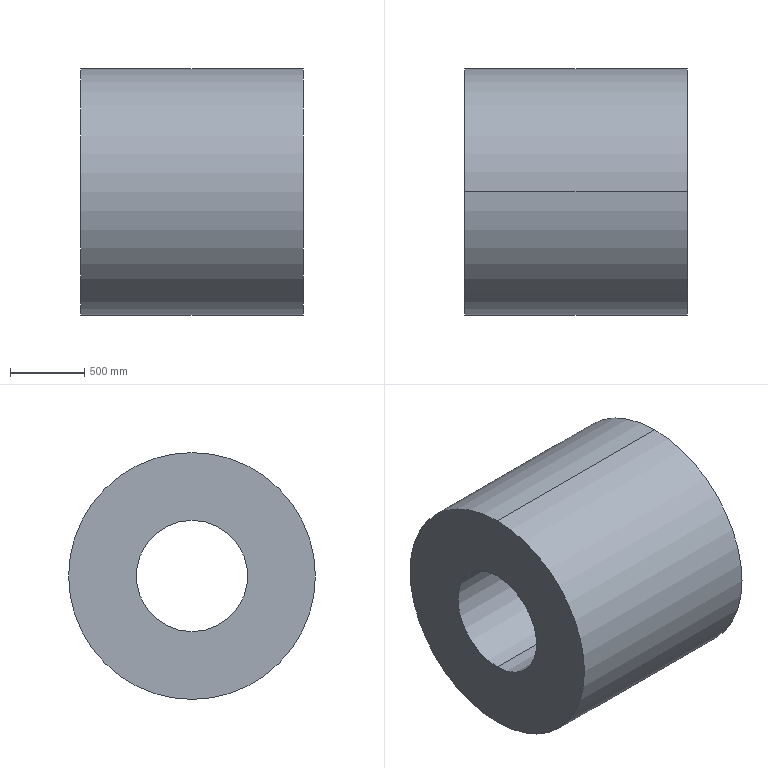Part | SolidWorks | features Extrusion 1 | 1 solid | 6 faces | box 1500 x 1660 x 1660 mm | volume 2583685068 mm3 | cylinder 4 | plane 2 | commonest cylinder face diameters 750 x2 1660 x2
STEP:
#1=CARTESIAN_POINT('',(1500.,0.,375.));
#2=VERTEX_POINT('',#1);
#3=CARTESIAN_POINT('',(1500.,0.,-375.));
#4=VERTEX_POINT('',#3);
#5=CARTESIAN_POINT('',(1500.,0.,0.));
#6=DIRECTION('',(1.,0.,0.));
#7=DIRECTION('',(0.,0.,-1.));
#8=AXIS2_PLACEMENT_3D('',#5,#6,#7);
#9=CIRCLE('',#8,375.);
#10=EDGE_CURVE('',#2,#4,#9,.T.);
#11=ORIENTED_EDGE('',*,*,#10,.T.);
#12=CARTESIAN_POINT('',(0.,0.,-375.));
#13=VERTEX_POINT('',#12);
#14=CARTESIAN_POINT('',(1500.,0.,-375.));
#15=DIRECTION('',(-1.,0.,0.));
#16=VECTOR('',#15,1000.);
#17=LINE('',#14,#16);
#18=EDGE_CURVE('',#4,#13,#17,.T.);
#19=ORIENTED_EDGE('',*,*,#18,.T.);
#20=CARTESIAN_POINT('',(0.,0.,375.));
#21=VERTEX_POINT('',#20);
#22=CARTESIAN_POINT('',(0.,0.,0.));
#23=DIRECTION('',(1.,0.,0.));
#24=DIRECTION('',(0.,0.,-1.));
#25=AXIS2_PLACEMENT_3D('',#22,#23,#24);
#26=CIRCLE('',#25,375.);
#27=EDGE_CURVE('',#21,#13,#26,.T.);
#28=ORIENTED_EDGE('',*,*,#27,.F.);
#29=CARTESIAN_POINT('',(1500.,0.,375.));
#30=DIRECTION('',(-1.,0.,0.));
#31=VECTOR('',#30,1000.);
#32=LINE('',#29,#31);
#33=EDGE_CURVE('',#2,#21,#32,.T.);
#34=ORIENTED_EDGE('',*,*,#33,.F.);
#35=EDGE_LOOP('',(#11,#19,#28,#34));
#36=FACE_OUTER_BOUND('',#35,.T.);
#37=CARTESIAN_POINT('',(1500.,0.,0.));
#38=DIRECTION('',(-1.,0.,0.));
#39=DIRECTION('',(0.,0.,1.));
#40=AXIS2_PLACEMENT_3D('',#37,#38,#39);
#41=CYLINDRICAL_SURFACE('',#40,375.);
#42=ADVANCED_FACE('',(#36),#41,.F.);
#43=CARTESIAN_POINT('',(1500.,0.,-830.));
#44=VERTEX_POINT('',#43);
#45=CARTESIAN_POINT('',(1500.,0.,830.));
#46=VERTEX_POINT('',#45);
#47=CARTESIAN_POINT('',(1500.,0.,0.));
#48=DIRECTION('',(1.,0.,0.));
#49=DIRECTION('',(0.,0.,-1.));
#50=AXIS2_PLACEMENT_3D('',#47,#48,#49);
#51=CIRCLE('',#50,830.);
#52=EDGE_CURVE('',#44,#46,#51,.T.);
#53=ORIENTED_EDGE('',*,*,#52,.F.);
#54=CARTESIAN_POINT('',(0.,0.,-830.));
#55=VERTEX_POINT('',#54);
#56=CARTESIAN_POINT('',(1500.,0.,-830.));
#57=DIRECTION('',(-1.,0.,0.));
#58=VECTOR('',#57,1000.);
#59=LINE('',#56,#58);
#60=EDGE_CURVE('',#44,#55,#59,.T.);
#61=ORIENTED_EDGE('',*,*,#60,.T.);
#62=CARTESIAN_POINT('',(0.,0.,830.));
#63=VERTEX_POINT('',#62);
#64=CARTESIAN_POINT('',(0.,0.,0.));
#65=DIRECTION('',(1.,0.,0.));
#66=DIRECTION('',(0.,0.,-1.));
#67=AXIS2_PLACEMENT_3D('',#64,#65,#66);
#68=CIRCLE('',#67,830.);
#69=EDGE_CURVE('',#55,#63,#68,.T.);
#70=ORIENTED_EDGE('',*,*,#69,.T.);
#71=CARTESIAN_POINT('',(1500.,0.,830.));
#72=DIRECTION('',(-1.,0.,0.));
#73=VECTOR('',#72,1000.);
#74=LINE('',#71,#73);
#75=EDGE_CURVE('',#46,#63,#74,.T.);
#76=ORIENTED_EDGE('',*,*,#75,.F.);
#77=EDGE_LOOP('',(#53,#61,#70,#76));
#78=FACE_OUTER_BOUND('',#77,.T.);
#79=CARTESIAN_POINT('',(1500.,0.,0.));
#80=DIRECTION('',(-1.,0.,0.));
#81=DIRECTION('',(0.,0.,1.));
#82=AXIS2_PLACEMENT_3D('',#79,#80,#81);
#83=CYLINDRICAL_SURFACE('',#82,830.);
#84=ADVANCED_FACE('',(#78),#83,.T.);
#85=CARTESIAN_POINT('',(1500.,0.,0.));
#86=DIRECTION('',(1.,0.,0.));
#87=DIRECTION('',(0.,0.,-1.));
#88=AXIS2_PLACEMENT_3D('',#85,#86,#87);
#89=CIRCLE('',#88,830.);
#90=EDGE_CURVE('',#46,#44,#89,.T.);
#91=ORIENTED_EDGE('',*,*,#90,.T.);
#92=ORIENTED_EDGE('',*,*,#52,.T.);
#93=EDGE_LOOP('',(#91,#92));
#94=FACE_OUTER_BOUND('',#93,.T.);
#95=ORIENTED_EDGE('',*,*,#10,.F.);
#96=CARTESIAN_POINT('',(1500.,0.,0.));
#97=DIRECTION('',(1.,0.,0.));
#98=DIRECTION('',(0.,0.,-1.));
#99=AXIS2_PLACEMENT_3D('',#96,#97,#98);
#100=CIRCLE('',#99,375.);
#101=EDGE_CURVE('',#4,#2,#100,.T.);
#102=ORIENTED_EDGE('',*,*,#101,.F.);
#103=EDGE_LOOP('',(#95,#102));
#104=FACE_BOUND('',#103,.T.);
#105=CARTESIAN_POINT('',(1500.,0.,0.));
#106=DIRECTION('',(1.,0.,0.));
#107=DIRECTION('',(0.,0.,-1.));
#108=AXIS2_PLACEMENT_3D('',#105,#106,#107);
#109=PLANE('',#108);
#110=ADVANCED_FACE('',(#94,#104),#109,.T.);
#111=CARTESIAN_POINT('',(0.,0.,0.));
#112=DIRECTION('',(1.,0.,0.));
#113=DIRECTION('',(0.,0.,-1.));
#114=AXIS2_PLACEMENT_3D('',#111,#112,#113);
#115=CIRCLE('',#114,830.);
#116=EDGE_CURVE('',#63,#55,#115,.T.);
#117=ORIENTED_EDGE('',*,*,#116,.F.);
#118=ORIENTED_EDGE('',*,*,#69,.F.);
#119=EDGE_LOOP('',(#117,#118));
#120=FACE_OUTER_BOUND('',#119,.T.);
#121=ORIENTED_EDGE('',*,*,#27,.T.);
#122=CARTESIAN_POINT('',(0.,0.,0.));
#123=DIRECTION('',(1.,0.,0.));
#124=DIRECTION('',(0.,0.,-1.));
#125=AXIS2_PLACEMENT_3D('',#122,#123,#124);
#126=CIRCLE('',#125,375.);
#127=EDGE_CURVE('',#13,#21,#126,.T.);
#128=ORIENTED_EDGE('',*,*,#127,.T.);
#129=EDGE_LOOP('',(#121,#128));
#130=FACE_BOUND('',#129,.T.);
#131=CARTESIAN_POINT('',(0.,0.,0.));
#132=DIRECTION('',(1.,0.,0.));
#133=DIRECTION('',(0.,0.,-1.));
#134=AXIS2_PLACEMENT_3D('',#131,#132,#133);
#135=PLANE('',#134);
#136=ADVANCED_FACE('',(#120,#130),#135,.F.);
#137=ORIENTED_EDGE('',*,*,#60,.F.);
#138=ORIENTED_EDGE('',*,*,#90,.F.);
#139=ORIENTED_EDGE('',*,*,#75,.T.);
#140=ORIENTED_EDGE('',*,*,#116,.T.);
#141=EDGE_LOOP('',(#137,#138,#139,#140));
#142=FACE_OUTER_BOUND('',#141,.T.);
#143=CARTESIAN_POINT('',(1500.,0.,0.));
#144=DIRECTION('',(-1.,0.,0.));
#145=DIRECTION('',(0.,0.,1.));
#146=AXIS2_PLACEMENT_3D('',#143,#144,#145);
#147=CYLINDRICAL_SURFACE('',#146,830.);
#148=ADVANCED_FACE('',(#142),#147,.T.);
#149=ORIENTED_EDGE('',*,*,#18,.F.);
#150=ORIENTED_EDGE('',*,*,#101,.T.);
#151=ORIENTED_EDGE('',*,*,#33,.T.);
#152=ORIENTED_EDGE('',*,*,#127,.F.);
#153=EDGE_LOOP('',(#149,#150,#151,#152));
#154=FACE_OUTER_BOUND('',#153,.T.);
#155=CARTESIAN_POINT('',(1500.,0.,0.));
#156=DIRECTION('',(-1.,0.,0.));
#157=DIRECTION('',(0.,0.,1.));
#158=AXIS2_PLACEMENT_3D('',#155,#156,#157);
#159=CYLINDRICAL_SURFACE('',#158,375.);
#160=ADVANCED_FACE('',(#154),#159,.F.);
#161=CLOSED_SHELL('',(#42,#84,#110,#136,#148,#160));
#162=MANIFOLD_SOLID_BREP('',#161);
#163=CARTESIAN_POINT('',(0.,0.,0.));
#164=DIRECTION('',(0.,0.,1.));
#165=DIRECTION('',(1.,0.,0.));
#166=AXIS2_PLACEMENT_3D('',#163,#164,#165);
#167=(LENGTH_UNIT()NAMED_UNIT(*)SI_UNIT(.MILLI.,.METRE.));
#168=UNCERTAINTY_MEASURE_WITH_UNIT(LENGTH_MEASURE(0.00001),#167,'','');
#169=(NAMED_UNIT(*)PLANE_ANGLE_UNIT()SI_UNIT($,.RADIAN.));
#170=(NAMED_UNIT(*)SI_UNIT($,.STERADIAN.)SOLID_ANGLE_UNIT());
#171=(GEOMETRIC_REPRESENTATION_CONTEXT(3)GLOBAL_UNCERTAINTY_ASSIGNED_CONTEXT((#168))GLOBAL_UNIT_ASSIGNED_CONTEXT((#167,#169,#170))REPRESENTATION_CONTEXT('',''));
#172=ADVANCED_BREP_SHAPE_REPRESENTATION('',(#162,#166),#171);